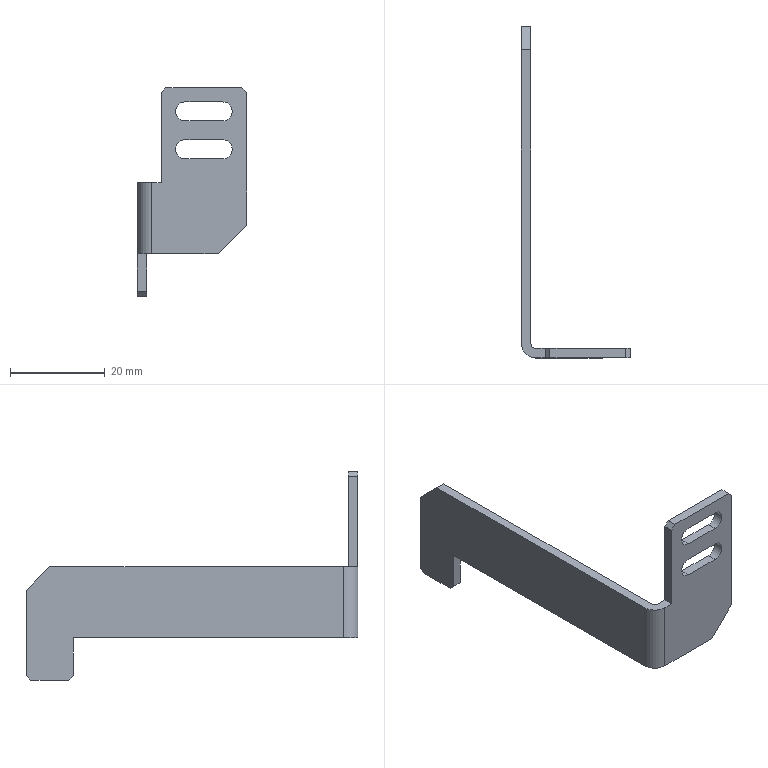Part | SolidWorks | features BaseBody 1 | 1 solid | 28 faces | box 23 x 70 x 44 mm | volume 3361 mm3 | plane 22 | cylinder 6 | commonest cylinder face diameters 4 x4 2 x1 6 x1
STEP:
#1=CARTESIAN_POINT('',(10.,-2.,16.5));
#2=VERTEX_POINT('',#1);
#3=CARTESIAN_POINT('',(9.,-2.,17.5));
#4=VERTEX_POINT('',#3);
#5=CARTESIAN_POINT('',(9.,-2.,17.5));
#6=DIRECTION('',(-0.7071,0.,0.7071));
#7=VECTOR('',#6,1000.);
#8=LINE('',#5,#7);
#9=EDGE_CURVE('',#2,#4,#8,.T.);
#10=ORIENTED_EDGE('',*,*,#9,.F.);
#11=CARTESIAN_POINT('',(10.,0.,16.5));
#12=VERTEX_POINT('',#11);
#13=CARTESIAN_POINT('',(10.,-2.,16.5));
#14=DIRECTION('',(0.,-1.,0.));
#15=VECTOR('',#14,1000.);
#16=LINE('',#13,#15);
#17=EDGE_CURVE('',#12,#2,#16,.T.);
#18=ORIENTED_EDGE('',*,*,#17,.F.);
#19=CARTESIAN_POINT('',(9.,0.,17.5));
#20=VERTEX_POINT('',#19);
#21=CARTESIAN_POINT('',(13.25,0.,13.25));
#22=DIRECTION('',(0.7071,0.,-0.7071));
#23=VECTOR('',#22,1000.);
#24=LINE('',#21,#23);
#25=EDGE_CURVE('',#20,#12,#24,.T.);
#26=ORIENTED_EDGE('',*,*,#25,.F.);
#27=CARTESIAN_POINT('',(9.,-2.,17.5));
#28=DIRECTION('',(0.,1.,0.));
#29=VECTOR('',#28,1000.);
#30=LINE('',#27,#29);
#31=EDGE_CURVE('',#4,#20,#30,.T.);
#32=ORIENTED_EDGE('',*,*,#31,.F.);
#33=EDGE_LOOP('',(#10,#18,#26,#32));
#34=FACE_OUTER_BOUND('',#33,.T.);
#35=CARTESIAN_POINT('',(9.,-2.,17.5));
#36=DIRECTION('',(-0.7071,0.,-0.7071));
#37=DIRECTION('',(-0.7071,0.,0.7071));
#38=AXIS2_PLACEMENT_3D('',#35,#36,#37);
#39=PLANE('',#38);
#40=ADVANCED_FACE('',(#34),#39,.F.);
#41=CARTESIAN_POINT('',(-7.,-2.,17.5));
#42=VERTEX_POINT('',#41);
#43=CARTESIAN_POINT('',(-8.,-2.,16.5));
#44=VERTEX_POINT('',#43);
#45=CARTESIAN_POINT('',(-8.,-2.,16.5));
#46=DIRECTION('',(-0.7071,0.,-0.7071));
#47=VECTOR('',#46,1000.);
#48=LINE('',#45,#47);
#49=EDGE_CURVE('',#42,#44,#48,.T.);
#50=ORIENTED_EDGE('',*,*,#49,.F.);
#51=CARTESIAN_POINT('',(-7.,0.,17.5));
#52=VERTEX_POINT('',#51);
#53=CARTESIAN_POINT('',(-7.,-2.,17.5));
#54=DIRECTION('',(0.,-1.,0.));
#55=VECTOR('',#54,1000.);
#56=LINE('',#53,#55);
#57=EDGE_CURVE('',#52,#42,#56,.T.);
#58=ORIENTED_EDGE('',*,*,#57,.F.);
#59=CARTESIAN_POINT('',(-8.,0.,16.5));
#60=VERTEX_POINT('',#59);
#61=CARTESIAN_POINT('',(-12.25,0.,12.25));
#62=DIRECTION('',(0.7071,0.,0.7071));
#63=VECTOR('',#62,1000.);
#64=LINE('',#61,#63);
#65=EDGE_CURVE('',#60,#52,#64,.T.);
#66=ORIENTED_EDGE('',*,*,#65,.F.);
#67=CARTESIAN_POINT('',(-8.,0.,16.5));
#68=DIRECTION('',(0.,1.,0.));
#69=VECTOR('',#68,1000.);
#70=LINE('',#67,#69);
#71=EDGE_CURVE('',#44,#60,#70,.T.);
#72=ORIENTED_EDGE('',*,*,#71,.F.);
#73=EDGE_LOOP('',(#50,#58,#66,#72));
#74=FACE_OUTER_BOUND('',#73,.T.);
#75=CARTESIAN_POINT('',(-8.,0.,16.5));
#76=DIRECTION('',(-0.7071,0.,0.7071));
#77=DIRECTION('',(0.,1.,0.));
#78=AXIS2_PLACEMENT_3D('',#75,#76,#77);
#79=PLANE('',#78);
#80=ADVANCED_FACE('',(#74),#79,.T.);
#81=CARTESIAN_POINT('',(-13.,59.,-26.5));
#82=VERTEX_POINT('',#81);
#83=CARTESIAN_POINT('',(-13.,58.,-25.5));
#84=VERTEX_POINT('',#83);
#85=CARTESIAN_POINT('',(-13.,58.,-25.5));
#86=DIRECTION('',(0.,-0.7071,0.7071));
#87=VECTOR('',#86,1000.);
#88=LINE('',#85,#87);
#89=EDGE_CURVE('',#82,#84,#88,.T.);
#90=ORIENTED_EDGE('',*,*,#89,.F.);
#91=CARTESIAN_POINT('',(-11.,59.,-26.5));
#92=VERTEX_POINT('',#91);
#93=CARTESIAN_POINT('',(-26.454,59.,-26.5));
#94=DIRECTION('',(-1.,0.,0.));
#95=VECTOR('',#94,1000.);
#96=LINE('',#93,#95);
#97=EDGE_CURVE('',#92,#82,#96,.T.);
#98=ORIENTED_EDGE('',*,*,#97,.F.);
#99=CARTESIAN_POINT('',(-11.,58.,-25.5));
#100=VERTEX_POINT('',#99);
#101=CARTESIAN_POINT('',(-11.,16.25,16.25));
#102=DIRECTION('',(0.,0.7071,-0.7071));
#103=VECTOR('',#102,1000.);
#104=LINE('',#101,#103);
#105=EDGE_CURVE('',#100,#92,#104,.T.);
#106=ORIENTED_EDGE('',*,*,#105,.F.);
#107=CARTESIAN_POINT('',(-26.454,58.,-25.5));
#108=DIRECTION('',(1.,0.,0.));
#109=VECTOR('',#108,1000.);
#110=LINE('',#107,#109);
#111=EDGE_CURVE('',#84,#100,#110,.T.);
#112=ORIENTED_EDGE('',*,*,#111,.F.);
#113=EDGE_LOOP('',(#90,#98,#106,#112));
#114=FACE_OUTER_BOUND('',#113,.T.);
#115=CARTESIAN_POINT('',(-26.454,58.,-25.5));
#116=DIRECTION('',(0.,0.7071,0.7071));
#117=DIRECTION('',(1.,0.,0.));
#118=AXIS2_PLACEMENT_3D('',#115,#116,#117);
#119=PLANE('',#118);
#120=ADVANCED_FACE('',(#114),#119,.F.);
#121=CARTESIAN_POINT('',(-13.,68.,-25.5));
#122=VERTEX_POINT('',#121);
#123=CARTESIAN_POINT('',(-13.,67.,-26.5));
#124=VERTEX_POINT('',#123);
#125=CARTESIAN_POINT('',(-13.,67.,-26.5));
#126=DIRECTION('',(0.,-0.7071,-0.7071));
#127=VECTOR('',#126,1000.);
#128=LINE('',#125,#127);
#129=EDGE_CURVE('',#122,#124,#128,.T.);
#130=ORIENTED_EDGE('',*,*,#129,.F.);
#131=CARTESIAN_POINT('',(-11.,68.,-25.5));
#132=VERTEX_POINT('',#131);
#133=CARTESIAN_POINT('',(-13.,68.,-25.5));
#134=DIRECTION('',(-1.,0.,0.));
#135=VECTOR('',#134,1000.);
#136=LINE('',#133,#135);
#137=EDGE_CURVE('',#132,#122,#136,.T.);
#138=ORIENTED_EDGE('',*,*,#137,.F.);
#139=CARTESIAN_POINT('',(-11.,67.,-26.5));
#140=VERTEX_POINT('',#139);
#141=CARTESIAN_POINT('',(-11.,46.75,-46.75));
#142=DIRECTION('',(0.,0.7071,0.7071));
#143=VECTOR('',#142,1000.);
#144=LINE('',#141,#143);
#145=EDGE_CURVE('',#140,#132,#144,.T.);
#146=ORIENTED_EDGE('',*,*,#145,.F.);
#147=CARTESIAN_POINT('',(-11.,67.,-26.5));
#148=DIRECTION('',(1.,0.,0.));
#149=VECTOR('',#148,1000.);
#150=LINE('',#147,#149);
#151=EDGE_CURVE('',#124,#140,#150,.T.);
#152=ORIENTED_EDGE('',*,*,#151,.F.);
#153=EDGE_LOOP('',(#130,#138,#146,#152));
#154=FACE_OUTER_BOUND('',#153,.T.);
#155=CARTESIAN_POINT('',(-26.454,67.,-26.5));
#156=DIRECTION('',(0.,0.7071,-0.7071));
#157=DIRECTION('',(-1.,0.,0.));
#158=AXIS2_PLACEMENT_3D('',#155,#156,#157);
#159=PLANE('',#158);
#160=ADVANCED_FACE('',(#154),#159,.T.);
#161=CARTESIAN_POINT('',(-3.,-2.,14.5));
#162=VERTEX_POINT('',#161);
#163=CARTESIAN_POINT('',(-3.,0.,14.5));
#164=VERTEX_POINT('',#163);
#165=CARTESIAN_POINT('',(-3.,-10.,14.5));
#166=DIRECTION('',(0.,1.,0.));
#167=VECTOR('',#166,1000.);
#168=LINE('',#165,#167);
#169=EDGE_CURVE('',#162,#164,#168,.T.);
#170=ORIENTED_EDGE('',*,*,#169,.T.);
#171=CARTESIAN_POINT('',(5.,0.,14.5));
#172=VERTEX_POINT('',#171);
#173=CARTESIAN_POINT('',(-3.,0.,14.5));
#174=DIRECTION('',(1.,0.,0.));
#175=VECTOR('',#174,1000.);
#176=LINE('',#173,#175);
#177=EDGE_CURVE('',#164,#172,#176,.T.);
#178=ORIENTED_EDGE('',*,*,#177,.T.);
#179=CARTESIAN_POINT('',(5.,-2.,14.5));
#180=VERTEX_POINT('',#179);
#181=CARTESIAN_POINT('',(5.,-10.,14.5));
#182=DIRECTION('',(0.,1.,0.));
#183=VECTOR('',#182,1000.);
#184=LINE('',#181,#183);
#185=EDGE_CURVE('',#180,#172,#184,.T.);
#186=ORIENTED_EDGE('',*,*,#185,.F.);
#187=CARTESIAN_POINT('',(0.,-2.,14.5));
#188=DIRECTION('',(1.,0.,0.));
#189=VECTOR('',#188,1000.);
#190=LINE('',#187,#189);
#191=EDGE_CURVE('',#162,#180,#190,.T.);
#192=ORIENTED_EDGE('',*,*,#191,.F.);
#193=EDGE_LOOP('',(#170,#178,#186,#192));
#194=FACE_OUTER_BOUND('',#193,.T.);
#195=CARTESIAN_POINT('',(-3.,-10.,14.5));
#196=DIRECTION('',(0.,0.,1.));
#197=DIRECTION('',(1.,0.,0.));
#198=AXIS2_PLACEMENT_3D('',#195,#196,#197);
#199=PLANE('',#198);
#200=ADVANCED_FACE('',(#194),#199,.F.);
#201=ORIENTED_EDGE('',*,*,#185,.T.);
#202=CARTESIAN_POINT('',(5.,0.,10.5));
#203=VERTEX_POINT('',#202);
#204=CARTESIAN_POINT('',(5.,0.,12.5));
#205=DIRECTION('',(0.,1.,0.));
#206=DIRECTION('',(0.,0.,1.));
#207=AXIS2_PLACEMENT_3D('',#204,#205,#206);
#208=CIRCLE('',#207,2.);
#209=EDGE_CURVE('',#172,#203,#208,.T.);
#210=ORIENTED_EDGE('',*,*,#209,.T.);
#211=CARTESIAN_POINT('',(5.,-2.,10.5));
#212=VERTEX_POINT('',#211);
#213=CARTESIAN_POINT('',(5.,-10.,10.5));
#214=DIRECTION('',(0.,1.,0.));
#215=VECTOR('',#214,1000.);
#216=LINE('',#213,#215);
#217=EDGE_CURVE('',#212,#203,#216,.T.);
#218=ORIENTED_EDGE('',*,*,#217,.F.);
#219=CARTESIAN_POINT('',(5.,-2.,12.5));
#220=DIRECTION('',(0.,1.,0.));
#221=DIRECTION('',(0.,0.,1.));
#222=AXIS2_PLACEMENT_3D('',#219,#220,#221);
#223=CIRCLE('',#222,2.);
#224=EDGE_CURVE('',#180,#212,#223,.T.);
#225=ORIENTED_EDGE('',*,*,#224,.F.);
#226=EDGE_LOOP('',(#201,#210,#218,#225));
#227=FACE_OUTER_BOUND('',#226,.T.);
#228=CARTESIAN_POINT('',(5.,-10.,12.5));
#229=DIRECTION('',(0.,1.,0.));
#230=DIRECTION('',(0.,0.,1.));
#231=AXIS2_PLACEMENT_3D('',#228,#229,#230);
#232=CYLINDRICAL_SURFACE('',#231,2.);
#233=ADVANCED_FACE('',(#227),#232,.F.);
#234=ORIENTED_EDGE('',*,*,#217,.T.);
#235=CARTESIAN_POINT('',(-3.,0.,10.5));
#236=VERTEX_POINT('',#235);
#237=CARTESIAN_POINT('',(-3.,0.,10.5));
#238=DIRECTION('',(-1.,0.,0.));
#239=VECTOR('',#238,1000.);
#240=LINE('',#237,#239);
#241=EDGE_CURVE('',#203,#236,#240,.T.);
#242=ORIENTED_EDGE('',*,*,#241,.T.);
#243=CARTESIAN_POINT('',(-3.,-2.,10.5));
#244=VERTEX_POINT('',#243);
#245=CARTESIAN_POINT('',(-3.,-10.,10.5));
#246=DIRECTION('',(0.,1.,0.));
#247=VECTOR('',#246,1000.);
#248=LINE('',#245,#247);
#249=EDGE_CURVE('',#244,#236,#248,.T.);
#250=ORIENTED_EDGE('',*,*,#249,.F.);
#251=CARTESIAN_POINT('',(0.,-2.,10.5));
#252=DIRECTION('',(-1.,0.,0.));
#253=VECTOR('',#252,1000.);
#254=LINE('',#251,#253);
#255=EDGE_CURVE('',#212,#244,#254,.T.);
#256=ORIENTED_EDGE('',*,*,#255,.F.);
#257=EDGE_LOOP('',(#234,#242,#250,#256));
#258=FACE_OUTER_BOUND('',#257,.T.);
#259=CARTESIAN_POINT('',(-3.,-10.,10.5));
#260=DIRECTION('',(0.,0.,-1.));
#261=DIRECTION('',(-1.,0.,0.));
#262=AXIS2_PLACEMENT_3D('',#259,#260,#261);
#263=PLANE('',#262);
#264=ADVANCED_FACE('',(#258),#263,.F.);
#265=ORIENTED_EDGE('',*,*,#249,.T.);
#266=CARTESIAN_POINT('',(-3.,0.,12.5));
#267=DIRECTION('',(0.,1.,0.));
#268=DIRECTION('',(0.,0.,1.));
#269=AXIS2_PLACEMENT_3D('',#266,#267,#268);
#270=CIRCLE('',#269,2.);
#271=EDGE_CURVE('',#236,#164,#270,.T.);
#272=ORIENTED_EDGE('',*,*,#271,.T.);
#273=ORIENTED_EDGE('',*,*,#169,.F.);
#274=CARTESIAN_POINT('',(-3.,-2.,12.5));
#275=DIRECTION('',(0.,1.,0.));
#276=DIRECTION('',(0.,0.,1.));
#277=AXIS2_PLACEMENT_3D('',#274,#275,#276);
#278=CIRCLE('',#277,2.);
#279=EDGE_CURVE('',#244,#162,#278,.T.);
#280=ORIENTED_EDGE('',*,*,#279,.F.);
#281=EDGE_LOOP('',(#265,#272,#273,#280));
#282=FACE_OUTER_BOUND('',#281,.T.);
#283=CARTESIAN_POINT('',(-3.,-10.,12.5));
#284=DIRECTION('',(0.,1.,0.));
#285=DIRECTION('',(0.,0.,1.));
#286=AXIS2_PLACEMENT_3D('',#283,#284,#285);
#287=CYLINDRICAL_SURFACE('',#286,2.);
#288=ADVANCED_FACE('',(#282),#287,.F.);
#289=CARTESIAN_POINT('',(-3.,-2.,6.5));
#290=VERTEX_POINT('',#289);
#291=CARTESIAN_POINT('',(-3.,0.,6.5));
#292=VERTEX_POINT('',#291);
#293=CARTESIAN_POINT('',(-3.,-10.,6.5));
#294=DIRECTION('',(0.,1.,0.));
#295=VECTOR('',#294,1000.);
#296=LINE('',#293,#295);
#297=EDGE_CURVE('',#290,#292,#296,.T.);
#298=ORIENTED_EDGE('',*,*,#297,.T.);
#299=CARTESIAN_POINT('',(5.,0.,6.5));
#300=VERTEX_POINT('',#299);
#301=CARTESIAN_POINT('',(-3.,0.,6.5));
#302=DIRECTION('',(1.,0.,0.));
#303=VECTOR('',#302,1000.);
#304=LINE('',#301,#303);
#305=EDGE_CURVE('',#292,#300,#304,.T.);
#306=ORIENTED_EDGE('',*,*,#305,.T.);
#307=CARTESIAN_POINT('',(5.,-2.,6.5));
#308=VERTEX_POINT('',#307);
#309=CARTESIAN_POINT('',(5.,-10.,6.5));
#310=DIRECTION('',(0.,1.,0.));
#311=VECTOR('',#310,1000.);
#312=LINE('',#309,#311);
#313=EDGE_CURVE('',#308,#300,#312,.T.);
#314=ORIENTED_EDGE('',*,*,#313,.F.);
#315=CARTESIAN_POINT('',(0.,-2.,6.5));
#316=DIRECTION('',(1.,0.,0.));
#317=VECTOR('',#316,1000.);
#318=LINE('',#315,#317);
#319=EDGE_CURVE('',#290,#308,#318,.T.);
#320=ORIENTED_EDGE('',*,*,#319,.F.);
#321=EDGE_LOOP('',(#298,#306,#314,#320));
#322=FACE_OUTER_BOUND('',#321,.T.);
#323=CARTESIAN_POINT('',(-3.,-10.,6.5));
#324=DIRECTION('',(0.,0.,1.));
#325=DIRECTION('',(1.,0.,0.));
#326=AXIS2_PLACEMENT_3D('',#323,#324,#325);
#327=PLANE('',#326);
#328=ADVANCED_FACE('',(#322),#327,.F.);
#329=ORIENTED_EDGE('',*,*,#313,.T.);
#330=CARTESIAN_POINT('',(5.,0.,2.5));
#331=VERTEX_POINT('',#330);
#332=CARTESIAN_POINT('',(5.,0.,4.5));
#333=DIRECTION('',(0.,1.,0.));
#334=DIRECTION('',(0.,0.,1.));
#335=AXIS2_PLACEMENT_3D('',#332,#333,#334);
#336=CIRCLE('',#335,2.);
#337=EDGE_CURVE('',#300,#331,#336,.T.);
#338=ORIENTED_EDGE('',*,*,#337,.T.);
#339=CARTESIAN_POINT('',(5.,-2.,2.5));
#340=VERTEX_POINT('',#339);
#341=CARTESIAN_POINT('',(5.,-10.,2.5));
#342=DIRECTION('',(0.,1.,0.));
#343=VECTOR('',#342,1000.);
#344=LINE('',#341,#343);
#345=EDGE_CURVE('',#340,#331,#344,.T.);
#346=ORIENTED_EDGE('',*,*,#345,.F.);
#347=CARTESIAN_POINT('',(5.,-2.,4.5));
#348=DIRECTION('',(0.,1.,0.));
#349=DIRECTION('',(0.,0.,1.));
#350=AXIS2_PLACEMENT_3D('',#347,#348,#349);
#351=CIRCLE('',#350,2.);
#352=EDGE_CURVE('',#308,#340,#351,.T.);
#353=ORIENTED_EDGE('',*,*,#352,.F.);
#354=EDGE_LOOP('',(#329,#338,#346,#353));
#355=FACE_OUTER_BOUND('',#354,.T.);
#356=CARTESIAN_POINT('',(5.,-10.,4.5));
#357=DIRECTION('',(0.,1.,0.));
#358=DIRECTION('',(0.,0.,1.));
#359=AXIS2_PLACEMENT_3D('',#356,#357,#358);
#360=CYLINDRICAL_SURFACE('',#359,2.);
#361=ADVANCED_FACE('',(#355),#360,.F.);
#362=ORIENTED_EDGE('',*,*,#345,.T.);
#363=CARTESIAN_POINT('',(-3.,0.,2.5));
#364=VERTEX_POINT('',#363);
#365=CARTESIAN_POINT('',(-3.,0.,2.5));
#366=DIRECTION('',(-1.,0.,0.));
#367=VECTOR('',#366,1000.);
#368=LINE('',#365,#367);
#369=EDGE_CURVE('',#331,#364,#368,.T.);
#370=ORIENTED_EDGE('',*,*,#369,.T.);
#371=CARTESIAN_POINT('',(-3.,-2.,2.5));
#372=VERTEX_POINT('',#371);
#373=CARTESIAN_POINT('',(-3.,-10.,2.5));
#374=DIRECTION('',(0.,1.,0.));
#375=VECTOR('',#374,1000.);
#376=LINE('',#373,#375);
#377=EDGE_CURVE('',#372,#364,#376,.T.);
#378=ORIENTED_EDGE('',*,*,#377,.F.);
#379=CARTESIAN_POINT('',(0.,-2.,2.5));
#380=DIRECTION('',(-1.,0.,0.));
#381=VECTOR('',#380,1000.);
#382=LINE('',#379,#381);
#383=EDGE_CURVE('',#340,#372,#382,.T.);
#384=ORIENTED_EDGE('',*,*,#383,.F.);
#385=EDGE_LOOP('',(#362,#370,#378,#384));
#386=FACE_OUTER_BOUND('',#385,.T.);
#387=CARTESIAN_POINT('',(-3.,-10.,2.5));
#388=DIRECTION('',(0.,0.,-1.));
#389=DIRECTION('',(-1.,0.,0.));
#390=AXIS2_PLACEMENT_3D('',#387,#388,#389);
#391=PLANE('',#390);
#392=ADVANCED_FACE('',(#386),#391,.F.);
#393=ORIENTED_EDGE('',*,*,#377,.T.);
#394=CARTESIAN_POINT('',(-3.,0.,4.5));
#395=DIRECTION('',(0.,1.,0.));
#396=DIRECTION('',(0.,0.,1.));
#397=AXIS2_PLACEMENT_3D('',#394,#395,#396);
#398=CIRCLE('',#397,2.);
#399=EDGE_CURVE('',#364,#292,#398,.T.);
#400=ORIENTED_EDGE('',*,*,#399,.T.);
#401=ORIENTED_EDGE('',*,*,#297,.F.);
#402=CARTESIAN_POINT('',(-3.,-2.,4.5));
#403=DIRECTION('',(0.,1.,0.));
#404=DIRECTION('',(0.,0.,1.));
#405=AXIS2_PLACEMENT_3D('',#402,#403,#404);
#406=CIRCLE('',#405,2.);
#407=EDGE_CURVE('',#372,#290,#406,.T.);
#408=ORIENTED_EDGE('',*,*,#407,.F.);
#409=EDGE_LOOP('',(#393,#400,#401,#408));
#410=FACE_OUTER_BOUND('',#409,.T.);
#411=CARTESIAN_POINT('',(-3.,-10.,4.5));
#412=DIRECTION('',(0.,1.,0.));
#413=DIRECTION('',(0.,0.,1.));
#414=AXIS2_PLACEMENT_3D('',#411,#412,#413);
#415=CYLINDRICAL_SURFACE('',#414,2.);
#416=ADVANCED_FACE('',(#410),#415,.F.);
#417=CARTESIAN_POINT('',(-13.,63.,-2.5));
#418=VERTEX_POINT('',#417);
#419=CARTESIAN_POINT('',(-13.,68.,-7.5));
#420=VERTEX_POINT('',#419);
#421=CARTESIAN_POINT('',(-13.,68.,-7.5));
#422=DIRECTION('',(0.,0.7071,-0.7071));
#423=VECTOR('',#422,1000.);
#424=LINE('',#421,#423);
#425=EDGE_CURVE('',#418,#420,#424,.T.);
#426=ORIENTED_EDGE('',*,*,#425,.F.);
#427=CARTESIAN_POINT('',(-11.,63.,-2.5));
#428=VERTEX_POINT('',#427);
#429=CARTESIAN_POINT('',(-8.,63.,-2.5));
#430=DIRECTION('',(-1.,0.,0.));
#431=VECTOR('',#430,1000.);
#432=LINE('',#429,#431);
#433=EDGE_CURVE('',#428,#418,#432,.T.);
#434=ORIENTED_EDGE('',*,*,#433,.F.);
#435=CARTESIAN_POINT('',(-11.,68.,-7.5));
#436=VERTEX_POINT('',#435);
#437=CARTESIAN_POINT('',(-11.,30.25,30.25));
#438=DIRECTION('',(0.,-0.7071,0.7071));
#439=VECTOR('',#438,1000.);
#440=LINE('',#437,#439);
#441=EDGE_CURVE('',#436,#428,#440,.T.);
#442=ORIENTED_EDGE('',*,*,#441,.F.);
#443=CARTESIAN_POINT('',(-13.,68.,-7.5));
#444=DIRECTION('',(1.,0.,0.));
#445=VECTOR('',#444,1000.);
#446=LINE('',#443,#445);
#447=EDGE_CURVE('',#420,#436,#446,.T.);
#448=ORIENTED_EDGE('',*,*,#447,.F.);
#449=EDGE_LOOP('',(#426,#434,#442,#448));
#450=FACE_OUTER_BOUND('',#449,.T.);
#451=CARTESIAN_POINT('',(-13.,68.,-7.5));
#452=DIRECTION('',(0.,-0.7071,-0.7071));
#453=DIRECTION('',(0.,-0.7071,0.7071));
#454=AXIS2_PLACEMENT_3D('',#451,#452,#453);
#455=PLANE('',#454);
#456=ADVANCED_FACE('',(#450),#455,.F.);
#457=CARTESIAN_POINT('',(-13.,58.,-17.5));
#458=VERTEX_POINT('',#457);
#459=CARTESIAN_POINT('',(-13.,58.,-17.5));
#460=DIRECTION('',(0.,0.,1.));
#461=VECTOR('',#460,1000.);
#462=LINE('',#459,#461);
#463=EDGE_CURVE('',#84,#458,#462,.T.);
#464=ORIENTED_EDGE('',*,*,#463,.F.);
#465=ORIENTED_EDGE('',*,*,#111,.T.);
#466=CARTESIAN_POINT('',(-11.,58.,-17.5));
#467=VERTEX_POINT('',#466);
#468=CARTESIAN_POINT('',(-11.,58.,-17.5));
#469=DIRECTION('',(0.,0.,-1.));
#470=VECTOR('',#469,1000.);
#471=LINE('',#468,#470);
#472=EDGE_CURVE('',#467,#100,#471,.T.);
#473=ORIENTED_EDGE('',*,*,#472,.F.);
#474=CARTESIAN_POINT('',(-26.454,58.,-17.5));
#475=DIRECTION('',(1.,0.,0.));
#476=VECTOR('',#475,1000.);
#477=LINE('',#474,#476);
#478=EDGE_CURVE('',#458,#467,#477,.T.);
#479=ORIENTED_EDGE('',*,*,#478,.F.);
#480=EDGE_LOOP('',(#464,#465,#473,#479));
#481=FACE_OUTER_BOUND('',#480,.T.);
#482=CARTESIAN_POINT('',(-26.454,58.,-17.5));
#483=DIRECTION('',(0.,-1.,0.));
#484=DIRECTION('',(0.,0.,-1.));
#485=AXIS2_PLACEMENT_3D('',#482,#483,#484);
#486=PLANE('',#485);
#487=ADVANCED_FACE('',(#481),#486,.T.);
#488=CARTESIAN_POINT('',(-13.,68.,-26.5));
#489=DIRECTION('',(0.,-1.,0.));
#490=VECTOR('',#489,1000.);
#491=LINE('',#488,#490);
#492=EDGE_CURVE('',#124,#82,#491,.T.);
#493=ORIENTED_EDGE('',*,*,#492,.F.);
#494=ORIENTED_EDGE('',*,*,#151,.T.);
#495=CARTESIAN_POINT('',(-11.,68.,-26.5));
#496=DIRECTION('',(0.,1.,0.));
#497=VECTOR('',#496,1000.);
#498=LINE('',#495,#497);
#499=EDGE_CURVE('',#92,#140,#498,.T.);
#500=ORIENTED_EDGE('',*,*,#499,.F.);
#501=ORIENTED_EDGE('',*,*,#97,.T.);
#502=EDGE_LOOP('',(#493,#494,#500,#501));
#503=FACE_OUTER_BOUND('',#502,.T.);
#504=CARTESIAN_POINT('',(-26.454,68.,-26.5));
#505=DIRECTION('',(0.,0.,-1.));
#506=DIRECTION('',(0.,-1.,0.));
#507=AXIS2_PLACEMENT_3D('',#504,#505,#506);
#508=PLANE('',#507);
#509=ADVANCED_FACE('',(#503),#508,.T.);
#510=CARTESIAN_POINT('',(4.,-2.,-17.5));
#511=VERTEX_POINT('',#510);
#512=CARTESIAN_POINT('',(10.,-2.,-11.5));
#513=VERTEX_POINT('',#512);
#514=CARTESIAN_POINT('',(10.,-2.,-11.5));
#515=DIRECTION('',(0.7071,0.,0.7071));
#516=VECTOR('',#515,1000.);
#517=LINE('',#514,#516);
#518=EDGE_CURVE('',#511,#513,#517,.T.);
#519=ORIENTED_EDGE('',*,*,#518,.F.);
#520=CARTESIAN_POINT('',(4.,0.,-17.5));
#521=VERTEX_POINT('',#520);
#522=CARTESIAN_POINT('',(4.,-2.,-17.5));
#523=DIRECTION('',(0.,-1.,0.));
#524=VECTOR('',#523,1000.);
#525=LINE('',#522,#524);
#526=EDGE_CURVE('',#521,#511,#525,.T.);
#527=ORIENTED_EDGE('',*,*,#526,.F.);
#528=CARTESIAN_POINT('',(10.,0.,-11.5));
#529=VERTEX_POINT('',#528);
#530=CARTESIAN_POINT('',(10.75,0.,-10.75));
#531=DIRECTION('',(-0.7071,0.,-0.7071));
#532=VECTOR('',#531,1000.);
#533=LINE('',#530,#532);
#534=EDGE_CURVE('',#529,#521,#533,.T.);
#535=ORIENTED_EDGE('',*,*,#534,.F.);
#536=CARTESIAN_POINT('',(10.,-2.,-11.5));
#537=DIRECTION('',(0.,1.,0.));
#538=VECTOR('',#537,1000.);
#539=LINE('',#536,#538);
#540=EDGE_CURVE('',#513,#529,#539,.T.);
#541=ORIENTED_EDGE('',*,*,#540,.F.);
#542=EDGE_LOOP('',(#519,#527,#535,#541));
#543=FACE_OUTER_BOUND('',#542,.T.);
#544=CARTESIAN_POINT('',(10.,-2.,-11.5));
#545=DIRECTION('',(-0.7071,0.,0.7071));
#546=DIRECTION('',(0.,1.,0.));
#547=AXIS2_PLACEMENT_3D('',#544,#545,#546);
#548=PLANE('',#547);
#549=ADVANCED_FACE('',(#543),#548,.F.);
#550=CARTESIAN_POINT('',(-8.,-2.,-2.5));
#551=VERTEX_POINT('',#550);
#552=CARTESIAN_POINT('',(-8.,-2.,17.5));
#553=DIRECTION('',(0.,0.,1.));
#554=VECTOR('',#553,1000.);
#555=LINE('',#552,#554);
#556=EDGE_CURVE('',#551,#44,#555,.T.);
#557=ORIENTED_EDGE('',*,*,#556,.T.);
#558=ORIENTED_EDGE('',*,*,#71,.T.);
#559=CARTESIAN_POINT('',(-8.,0.,-2.5));
#560=VERTEX_POINT('',#559);
#561=CARTESIAN_POINT('',(-8.,0.,0.));
#562=DIRECTION('',(0.,0.,-1.));
#563=VECTOR('',#562,1000.);
#564=LINE('',#561,#563);
#565=EDGE_CURVE('',#60,#560,#564,.T.);
#566=ORIENTED_EDGE('',*,*,#565,.T.);
#567=CARTESIAN_POINT('',(-8.,68.,-2.5));
#568=DIRECTION('',(0.,-1.,0.));
#569=VECTOR('',#568,1000.);
#570=LINE('',#567,#569);
#571=EDGE_CURVE('',#560,#551,#570,.T.);
#572=ORIENTED_EDGE('',*,*,#571,.T.);
#573=EDGE_LOOP('',(#557,#558,#566,#572));
#574=FACE_OUTER_BOUND('',#573,.T.);
#575=CARTESIAN_POINT('',(-8.,0.,0.));
#576=DIRECTION('',(1.,0.,0.));
#577=DIRECTION('',(0.,1.,0.));
#578=AXIS2_PLACEMENT_3D('',#575,#576,#577);
#579=PLANE('',#578);
#580=ADVANCED_FACE('',(#574),#579,.F.);
#581=CARTESIAN_POINT('',(-11.,68.,-17.5));
#582=DIRECTION('',(0.,0.,-1.));
#583=VECTOR('',#582,1000.);
#584=LINE('',#581,#583);
#585=EDGE_CURVE('',#436,#132,#584,.T.);
#586=ORIENTED_EDGE('',*,*,#585,.T.);
#587=ORIENTED_EDGE('',*,*,#137,.T.);
#588=CARTESIAN_POINT('',(-13.,68.,0.));
#589=DIRECTION('',(0.,0.,-1.));
#590=VECTOR('',#589,1000.);
#591=LINE('',#588,#590);
#592=EDGE_CURVE('',#420,#122,#591,.T.);
#593=ORIENTED_EDGE('',*,*,#592,.F.);
#594=ORIENTED_EDGE('',*,*,#447,.T.);
#595=EDGE_LOOP('',(#586,#587,#593,#594));
#596=FACE_OUTER_BOUND('',#595,.T.);
#597=CARTESIAN_POINT('',(-13.,68.,-17.5));
#598=DIRECTION('',(0.,-1.,0.));
#599=DIRECTION('',(0.,0.,-1.));
#600=AXIS2_PLACEMENT_3D('',#597,#598,#599);
#601=PLANE('',#600);
#602=ADVANCED_FACE('',(#596),#601,.F.);
#603=ORIENTED_EDGE('',*,*,#499,.T.);
#604=ORIENTED_EDGE('',*,*,#145,.T.);
#605=ORIENTED_EDGE('',*,*,#585,.F.);
#606=ORIENTED_EDGE('',*,*,#441,.T.);
#607=CARTESIAN_POINT('',(-11.,1.,-2.5));
#608=VERTEX_POINT('',#607);
#609=CARTESIAN_POINT('',(-11.,0.,-2.5));
#610=DIRECTION('',(0.,1.,0.));
#611=VECTOR('',#610,1000.);
#612=LINE('',#609,#611);
#613=EDGE_CURVE('',#608,#428,#612,.T.);
#614=ORIENTED_EDGE('',*,*,#613,.F.);
#615=CARTESIAN_POINT('',(-11.,1.,-17.5));
#616=VERTEX_POINT('',#615);
#617=CARTESIAN_POINT('',(-11.,1.,-17.5));
#618=DIRECTION('',(0.,0.,1.));
#619=VECTOR('',#618,1000.);
#620=LINE('',#617,#619);
#621=EDGE_CURVE('',#616,#608,#620,.T.);
#622=ORIENTED_EDGE('',*,*,#621,.F.);
#623=CARTESIAN_POINT('',(-11.,0.,-17.5));
#624=DIRECTION('',(0.,-1.,0.));
#625=VECTOR('',#624,1000.);
#626=LINE('',#623,#625);
#627=EDGE_CURVE('',#467,#616,#626,.T.);
#628=ORIENTED_EDGE('',*,*,#627,.F.);
#629=ORIENTED_EDGE('',*,*,#472,.T.);
#630=ORIENTED_EDGE('',*,*,#105,.T.);
#631=EDGE_LOOP('',(#603,#604,#605,#606,#614,#622,#628,#629,#630));
#632=FACE_OUTER_BOUND('',#631,.T.);
#633=CARTESIAN_POINT('',(-11.,0.,0.));
#634=DIRECTION('',(1.,0.,0.));
#635=DIRECTION('',(0.,1.,0.));
#636=AXIS2_PLACEMENT_3D('',#633,#634,#635);
#637=PLANE('',#636);
#638=ADVANCED_FACE('',(#632),#637,.T.);
#639=ORIENTED_EDGE('',*,*,#592,.T.);
#640=ORIENTED_EDGE('',*,*,#129,.T.);
#641=ORIENTED_EDGE('',*,*,#492,.T.);
#642=ORIENTED_EDGE('',*,*,#89,.T.);
#643=ORIENTED_EDGE('',*,*,#463,.T.);
#644=CARTESIAN_POINT('',(-13.,1.,-17.5));
#645=VERTEX_POINT('',#644);
#646=CARTESIAN_POINT('',(-13.,0.,-17.5));
#647=DIRECTION('',(0.,-1.,0.));
#648=VECTOR('',#647,1000.);
#649=LINE('',#646,#648);
#650=EDGE_CURVE('',#458,#645,#649,.T.);
#651=ORIENTED_EDGE('',*,*,#650,.T.);
#652=CARTESIAN_POINT('',(-13.,1.,-2.5));
#653=VERTEX_POINT('',#652);
#654=CARTESIAN_POINT('',(-13.,1.,-17.5));
#655=DIRECTION('',(0.,0.,-1.));
#656=VECTOR('',#655,1000.);
#657=LINE('',#654,#656);
#658=EDGE_CURVE('',#653,#645,#657,.T.);
#659=ORIENTED_EDGE('',*,*,#658,.F.);
#660=CARTESIAN_POINT('',(-13.,68.,-2.5));
#661=DIRECTION('',(0.,-1.,0.));
#662=VECTOR('',#661,1000.);
#663=LINE('',#660,#662);
#664=EDGE_CURVE('',#418,#653,#663,.T.);
#665=ORIENTED_EDGE('',*,*,#664,.F.);
#666=ORIENTED_EDGE('',*,*,#425,.T.);
#667=EDGE_LOOP('',(#639,#640,#641,#642,#643,#651,#659,#665,#666));
#668=FACE_OUTER_BOUND('',#667,.T.);
#669=CARTESIAN_POINT('',(-13.,0.,0.));
#670=DIRECTION('',(1.,0.,0.));
#671=DIRECTION('',(0.,1.,0.));
#672=AXIS2_PLACEMENT_3D('',#669,#670,#671);
#673=PLANE('',#672);
#674=ADVANCED_FACE('',(#668),#673,.F.);
#675=ORIENTED_EDGE('',*,*,#621,.T.);
#676=CARTESIAN_POINT('',(-10.,0.,-2.5));
#677=VERTEX_POINT('',#676);
#678=CARTESIAN_POINT('',(-10.,1.,-2.5));
#679=DIRECTION('',(0.,0.,1.));
#680=DIRECTION('',(-1.,0.,0.));
#681=AXIS2_PLACEMENT_3D('',#678,#679,#680);
#682=CIRCLE('',#681,1.);
#683=EDGE_CURVE('',#608,#677,#682,.T.);
#684=ORIENTED_EDGE('',*,*,#683,.T.);
#685=CARTESIAN_POINT('',(-10.,0.,-17.5));
#686=VERTEX_POINT('',#685);
#687=CARTESIAN_POINT('',(-10.,0.,-17.5));
#688=DIRECTION('',(0.,0.,1.));
#689=VECTOR('',#688,1000.);
#690=LINE('',#687,#689);
#691=EDGE_CURVE('',#686,#677,#690,.T.);
#692=ORIENTED_EDGE('',*,*,#691,.F.);
#693=CARTESIAN_POINT('',(-10.,1.,-17.5));
#694=DIRECTION('',(0.,0.,-1.));
#695=DIRECTION('',(1.,0.,0.));
#696=AXIS2_PLACEMENT_3D('',#693,#694,#695);
#697=CIRCLE('',#696,1.);
#698=EDGE_CURVE('',#686,#616,#697,.T.);
#699=ORIENTED_EDGE('',*,*,#698,.T.);
#700=EDGE_LOOP('',(#675,#684,#692,#699));
#701=FACE_OUTER_BOUND('',#700,.T.);
#702=CARTESIAN_POINT('',(-10.,1.,17.5));
#703=DIRECTION('',(0.,0.,1.));
#704=DIRECTION('',(-1.,0.,0.));
#705=AXIS2_PLACEMENT_3D('',#702,#703,#704);
#706=CYLINDRICAL_SURFACE('',#705,1.);
#707=ADVANCED_FACE('',(#701),#706,.F.);
#708=CARTESIAN_POINT('',(-10.,-2.,-2.5));
#709=VERTEX_POINT('',#708);
#710=CARTESIAN_POINT('',(-10.,1.,-2.5));
#711=DIRECTION('',(0.,0.,1.));
#712=DIRECTION('',(-1.,0.,0.));
#713=AXIS2_PLACEMENT_3D('',#710,#711,#712);
#714=CIRCLE('',#713,3.);
#715=EDGE_CURVE('',#653,#709,#714,.T.);
#716=ORIENTED_EDGE('',*,*,#715,.F.);
#717=ORIENTED_EDGE('',*,*,#658,.T.);
#718=CARTESIAN_POINT('',(-10.,-2.,-17.5));
#719=VERTEX_POINT('',#718);
#720=CARTESIAN_POINT('',(-10.,1.,-17.5));
#721=DIRECTION('',(0.,0.,-1.));
#722=DIRECTION('',(1.,0.,0.));
#723=AXIS2_PLACEMENT_3D('',#720,#721,#722);
#724=CIRCLE('',#723,3.);
#725=EDGE_CURVE('',#719,#645,#724,.T.);
#726=ORIENTED_EDGE('',*,*,#725,.F.);
#727=CARTESIAN_POINT('',(-10.,-2.,-17.5));
#728=DIRECTION('',(0.,0.,1.));
#729=VECTOR('',#728,1000.);
#730=LINE('',#727,#729);
#731=EDGE_CURVE('',#719,#709,#730,.T.);
#732=ORIENTED_EDGE('',*,*,#731,.T.);
#733=EDGE_LOOP('',(#716,#717,#726,#732));
#734=FACE_OUTER_BOUND('',#733,.T.);
#735=CARTESIAN_POINT('',(-10.,1.,17.5));
#736=DIRECTION('',(0.,0.,1.));
#737=DIRECTION('',(-1.,0.,0.));
#738=AXIS2_PLACEMENT_3D('',#735,#736,#737);
#739=CYLINDRICAL_SURFACE('',#738,3.);
#740=ADVANCED_FACE('',(#734),#739,.T.);
#741=ORIENTED_EDGE('',*,*,#399,.F.);
#742=ORIENTED_EDGE('',*,*,#369,.F.);
#743=ORIENTED_EDGE('',*,*,#337,.F.);
#744=ORIENTED_EDGE('',*,*,#305,.F.);
#745=EDGE_LOOP('',(#741,#742,#743,#744));
#746=FACE_BOUND('',#745,.T.);
#747=ORIENTED_EDGE('',*,*,#271,.F.);
#748=ORIENTED_EDGE('',*,*,#241,.F.);
#749=ORIENTED_EDGE('',*,*,#209,.F.);
#750=ORIENTED_EDGE('',*,*,#177,.F.);
#751=EDGE_LOOP('',(#747,#748,#749,#750));
#752=FACE_BOUND('',#751,.T.);
#753=ORIENTED_EDGE('',*,*,#565,.F.);
#754=ORIENTED_EDGE('',*,*,#65,.T.);
#755=CARTESIAN_POINT('',(-10.,0.,17.5));
#756=DIRECTION('',(1.,0.,0.));
#757=VECTOR('',#756,1000.);
#758=LINE('',#755,#757);
#759=EDGE_CURVE('',#52,#20,#758,.T.);
#760=ORIENTED_EDGE('',*,*,#759,.T.);
#761=ORIENTED_EDGE('',*,*,#25,.T.);
#762=CARTESIAN_POINT('',(10.,0.,-17.5));
#763=DIRECTION('',(0.,0.,-1.));
#764=VECTOR('',#763,1000.);
#765=LINE('',#762,#764);
#766=EDGE_CURVE('',#12,#529,#765,.T.);
#767=ORIENTED_EDGE('',*,*,#766,.T.);
#768=ORIENTED_EDGE('',*,*,#534,.T.);
#769=CARTESIAN_POINT('',(-10.,0.,-17.5));
#770=DIRECTION('',(-1.,0.,0.));
#771=VECTOR('',#770,1000.);
#772=LINE('',#769,#771);
#773=EDGE_CURVE('',#521,#686,#772,.T.);
#774=ORIENTED_EDGE('',*,*,#773,.T.);
#775=ORIENTED_EDGE('',*,*,#691,.T.);
#776=CARTESIAN_POINT('',(0.,0.,-2.5));
#777=DIRECTION('',(-1.,0.,0.));
#778=VECTOR('',#777,1000.);
#779=LINE('',#776,#778);
#780=EDGE_CURVE('',#560,#677,#779,.T.);
#781=ORIENTED_EDGE('',*,*,#780,.F.);
#782=EDGE_LOOP('',(#753,#754,#760,#761,#767,#768,#774,#775,#781));
#783=FACE_OUTER_BOUND('',#782,.T.);
#784=CARTESIAN_POINT('',(0.,0.,0.));
#785=DIRECTION('',(0.,1.,0.));
#786=DIRECTION('',(1.,0.,0.));
#787=AXIS2_PLACEMENT_3D('',#784,#785,#786);
#788=PLANE('',#787);
#789=ADVANCED_FACE('',(#746,#752,#783),#788,.T.);
#790=ORIENTED_EDGE('',*,*,#383,.T.);
#791=ORIENTED_EDGE('',*,*,#407,.T.);
#792=ORIENTED_EDGE('',*,*,#319,.T.);
#793=ORIENTED_EDGE('',*,*,#352,.T.);
#794=EDGE_LOOP('',(#790,#791,#792,#793));
#795=FACE_BOUND('',#794,.T.);
#796=ORIENTED_EDGE('',*,*,#255,.T.);
#797=ORIENTED_EDGE('',*,*,#279,.T.);
#798=ORIENTED_EDGE('',*,*,#191,.T.);
#799=ORIENTED_EDGE('',*,*,#224,.T.);
#800=EDGE_LOOP('',(#796,#797,#798,#799));
#801=FACE_BOUND('',#800,.T.);
#802=CARTESIAN_POINT('',(-10.,-2.,17.5));
#803=DIRECTION('',(1.,0.,0.));
#804=VECTOR('',#803,1000.);
#805=LINE('',#802,#804);
#806=EDGE_CURVE('',#42,#4,#805,.T.);
#807=ORIENTED_EDGE('',*,*,#806,.F.);
#808=ORIENTED_EDGE('',*,*,#49,.T.);
#809=ORIENTED_EDGE('',*,*,#556,.F.);
#810=CARTESIAN_POINT('',(-8.,-2.,-2.5));
#811=DIRECTION('',(-1.,0.,0.));
#812=VECTOR('',#811,1000.);
#813=LINE('',#810,#812);
#814=EDGE_CURVE('',#551,#709,#813,.T.);
#815=ORIENTED_EDGE('',*,*,#814,.T.);
#816=ORIENTED_EDGE('',*,*,#731,.F.);
#817=CARTESIAN_POINT('',(-10.,-2.,-17.5));
#818=DIRECTION('',(-1.,0.,0.));
#819=VECTOR('',#818,1000.);
#820=LINE('',#817,#819);
#821=EDGE_CURVE('',#511,#719,#820,.T.);
#822=ORIENTED_EDGE('',*,*,#821,.F.);
#823=ORIENTED_EDGE('',*,*,#518,.T.);
#824=CARTESIAN_POINT('',(10.,-2.,-17.5));
#825=DIRECTION('',(0.,0.,-1.));
#826=VECTOR('',#825,1000.);
#827=LINE('',#824,#826);
#828=EDGE_CURVE('',#2,#513,#827,.T.);
#829=ORIENTED_EDGE('',*,*,#828,.F.);
#830=ORIENTED_EDGE('',*,*,#9,.T.);
#831=EDGE_LOOP('',(#807,#808,#809,#815,#816,#822,#823,#829,#830));
#832=FACE_OUTER_BOUND('',#831,.T.);
#833=CARTESIAN_POINT('',(0.,-2.,0.));
#834=DIRECTION('',(0.,1.,0.));
#835=DIRECTION('',(1.,0.,0.));
#836=AXIS2_PLACEMENT_3D('',#833,#834,#835);
#837=PLANE('',#836);
#838=ADVANCED_FACE('',(#795,#801,#832),#837,.F.);
#839=ORIENTED_EDGE('',*,*,#773,.F.);
#840=ORIENTED_EDGE('',*,*,#526,.T.);
#841=ORIENTED_EDGE('',*,*,#821,.T.);
#842=ORIENTED_EDGE('',*,*,#725,.T.);
#843=ORIENTED_EDGE('',*,*,#650,.F.);
#844=ORIENTED_EDGE('',*,*,#478,.T.);
#845=ORIENTED_EDGE('',*,*,#627,.T.);
#846=ORIENTED_EDGE('',*,*,#698,.F.);
#847=EDGE_LOOP('',(#839,#840,#841,#842,#843,#844,#845,#846));
#848=FACE_OUTER_BOUND('',#847,.T.);
#849=CARTESIAN_POINT('',(-10.,-2.,-17.5));
#850=DIRECTION('',(0.,0.,-1.));
#851=DIRECTION('',(0.,-1.,0.));
#852=AXIS2_PLACEMENT_3D('',#849,#850,#851);
#853=PLANE('',#852);
#854=ADVANCED_FACE('',(#848),#853,.T.);
#855=ORIENTED_EDGE('',*,*,#759,.F.);
#856=ORIENTED_EDGE('',*,*,#57,.T.);
#857=ORIENTED_EDGE('',*,*,#806,.T.);
#858=ORIENTED_EDGE('',*,*,#31,.T.);
#859=EDGE_LOOP('',(#855,#856,#857,#858));
#860=FACE_OUTER_BOUND('',#859,.T.);
#861=CARTESIAN_POINT('',(-10.,-2.,17.5));
#862=DIRECTION('',(0.,0.,1.));
#863=DIRECTION('',(1.,0.,0.));
#864=AXIS2_PLACEMENT_3D('',#861,#862,#863);
#865=PLANE('',#864);
#866=ADVANCED_FACE('',(#860),#865,.T.);
#867=ORIENTED_EDGE('',*,*,#766,.F.);
#868=ORIENTED_EDGE('',*,*,#17,.T.);
#869=ORIENTED_EDGE('',*,*,#828,.T.);
#870=ORIENTED_EDGE('',*,*,#540,.T.);
#871=EDGE_LOOP('',(#867,#868,#869,#870));
#872=FACE_OUTER_BOUND('',#871,.T.);
#873=CARTESIAN_POINT('',(10.,-2.,-17.5));
#874=DIRECTION('',(1.,0.,0.));
#875=DIRECTION('',(0.,0.,-1.));
#876=AXIS2_PLACEMENT_3D('',#873,#874,#875);
#877=PLANE('',#876);
#878=ADVANCED_FACE('',(#872),#877,.T.);
#879=ORIENTED_EDGE('',*,*,#780,.T.);
#880=ORIENTED_EDGE('',*,*,#683,.F.);
#881=ORIENTED_EDGE('',*,*,#613,.T.);
#882=ORIENTED_EDGE('',*,*,#433,.T.);
#883=ORIENTED_EDGE('',*,*,#664,.T.);
#884=ORIENTED_EDGE('',*,*,#715,.T.);
#885=ORIENTED_EDGE('',*,*,#814,.F.);
#886=ORIENTED_EDGE('',*,*,#571,.F.);
#887=EDGE_LOOP('',(#879,#880,#881,#882,#883,#884,#885,#886));
#888=FACE_OUTER_BOUND('',#887,.T.);
#889=CARTESIAN_POINT('',(-8.,68.,-2.5));
#890=DIRECTION('',(0.,0.,-1.));
#891=DIRECTION('',(-1.,0.,0.));
#892=AXIS2_PLACEMENT_3D('',#889,#890,#891);
#893=PLANE('',#892);
#894=ADVANCED_FACE('',(#888),#893,.F.);
#895=CLOSED_SHELL('',(#40,#80,#120,#160,#200,#233,#264,#288,#328,#361,#392,#416,#456,#487,#509,#549,#580,#602,#638,#674,#707,#740,#789,#838,#854,#866,#878,#894));
#896=MANIFOLD_SOLID_BREP('',#895);
#897=CARTESIAN_POINT('',(0.,0.,0.));
#898=DIRECTION('',(0.,0.,1.));
#899=DIRECTION('',(1.,0.,0.));
#900=AXIS2_PLACEMENT_3D('',#897,#898,#899);
#901=(LENGTH_UNIT()NAMED_UNIT(*)SI_UNIT(.MILLI.,.METRE.));
#902=UNCERTAINTY_MEASURE_WITH_UNIT(LENGTH_MEASURE(0.00001),#901,'','');
#903=(NAMED_UNIT(*)PLANE_ANGLE_UNIT()SI_UNIT($,.RADIAN.));
#904=(NAMED_UNIT(*)SI_UNIT($,.STERADIAN.)SOLID_ANGLE_UNIT());
#905=(GEOMETRIC_REPRESENTATION_CONTEXT(3)GLOBAL_UNCERTAINTY_ASSIGNED_CONTEXT((#902))GLOBAL_UNIT_ASSIGNED_CONTEXT((#901,#903,#904))REPRESENTATION_CONTEXT('',''));
#906=ADVANCED_BREP_SHAPE_REPRESENTATION('',(#896,#900),#905);